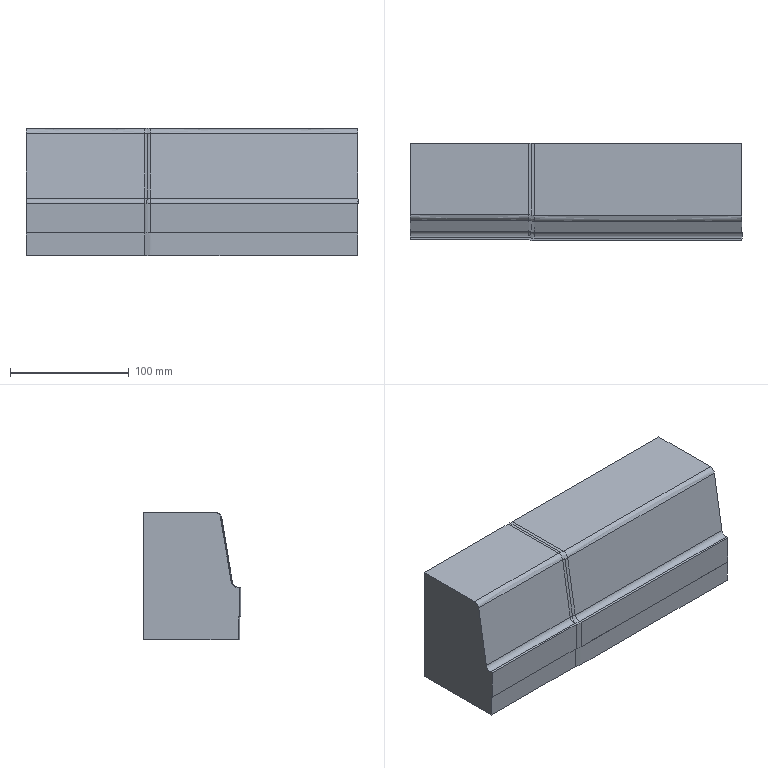Part | NX | features solid 2 | 1 solid | 39 faces | box 280 x 82.143 x 107.133 mm | volume 2215544 mm3 | plane 15 | spline 12 | cylinder 9 | cone 3 | commonest cylinder face diameters 12 x4 10 x2 20 x2 14 x1